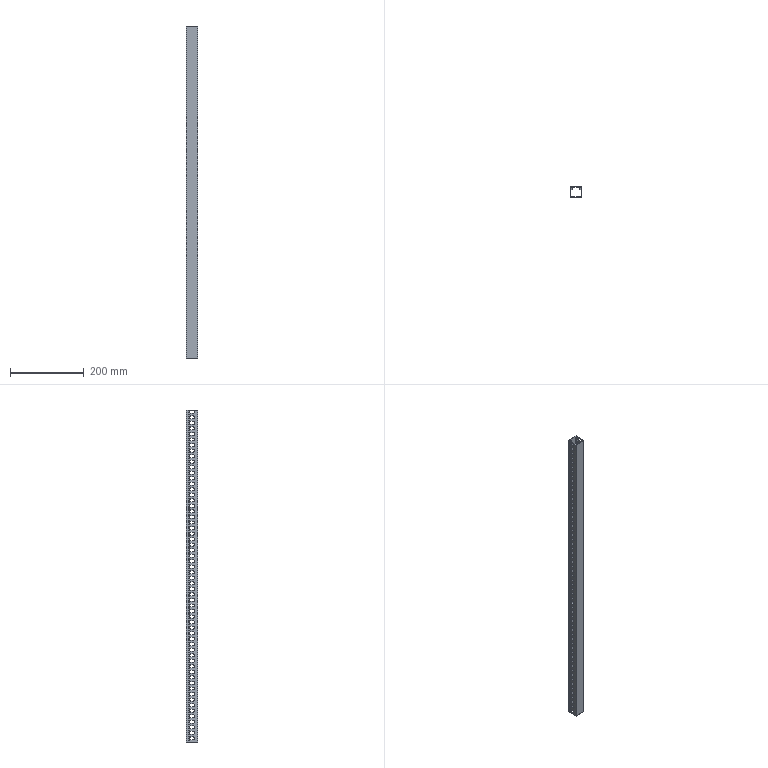Part | SolidWorks | features BaseBody 1 | 1 solid | 506 faces | box 30 x 30 x 900 mm | volume 110608 mm3 | plane 266 | cylinder 240 | commonest cylinder face diameters 8 x240